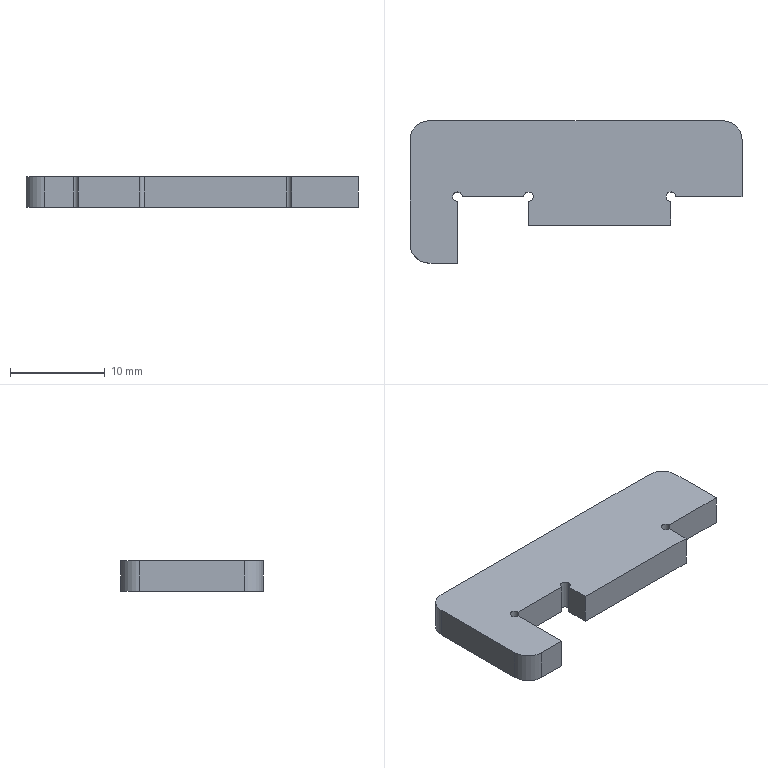Part | SolidWorks | features Fillet 1, FlatPattern 1, SMBaseFlange 1, SheetMetal 1 | 1 solid | 19 faces | box 35 x 15 x 3.2 mm | volume 1138 mm3 | plane 12 | cylinder 7 | commonest cylinder face diameters 1 x4 4 x3
STEP:
#1=CARTESIAN_POINT('',(47.21,-235.,-3.2));
#2=VERTEX_POINT('',#1);
#3=CARTESIAN_POINT('',(48.21,-235.,-3.2));
#4=VERTEX_POINT('',#3);
#5=CARTESIAN_POINT('',(47.71,-235.,-3.2));
#6=DIRECTION('',(0.,0.,-1.));
#7=DIRECTION('',(1.,0.,0.));
#8=AXIS2_PLACEMENT_3D('',#5,#6,#7);
#9=CIRCLE('',#8,0.5);
#10=EDGE_CURVE('',#2,#4,#9,.T.);
#11=ORIENTED_EDGE('',*,*,#10,.T.);
#12=CARTESIAN_POINT('',(48.21,-235.,0.));
#13=VERTEX_POINT('',#12);
#14=CARTESIAN_POINT('',(48.21,-235.,-3.2));
#15=DIRECTION('',(0.,0.,1.));
#16=VECTOR('',#15,1000.);
#17=LINE('',#14,#16);
#18=EDGE_CURVE('',#4,#13,#17,.T.);
#19=ORIENTED_EDGE('',*,*,#18,.T.);
#20=CARTESIAN_POINT('',(47.21,-235.,0.));
#21=VERTEX_POINT('',#20);
#22=CARTESIAN_POINT('',(47.71,-235.,0.));
#23=DIRECTION('',(0.,0.,-1.));
#24=DIRECTION('',(1.,0.,0.));
#25=AXIS2_PLACEMENT_3D('',#22,#23,#24);
#26=CIRCLE('',#25,0.5);
#27=EDGE_CURVE('',#21,#13,#26,.T.);
#28=ORIENTED_EDGE('',*,*,#27,.F.);
#29=CARTESIAN_POINT('',(47.21,-235.,-3.2));
#30=DIRECTION('',(0.,0.,1.));
#31=VECTOR('',#30,1000.);
#32=LINE('',#29,#31);
#33=EDGE_CURVE('',#2,#21,#32,.T.);
#34=ORIENTED_EDGE('',*,*,#33,.F.);
#35=EDGE_LOOP('',(#11,#19,#28,#34));
#36=FACE_OUTER_BOUND('',#35,.T.);
#37=CARTESIAN_POINT('',(47.71,-235.,-3.2));
#38=DIRECTION('',(0.,0.,1.));
#39=DIRECTION('',(1.,0.,0.));
#40=AXIS2_PLACEMENT_3D('',#37,#38,#39);
#41=CYLINDRICAL_SURFACE('',#40,0.5);
#42=ADVANCED_FACE('',(#36),#41,.F.);
#43=CARTESIAN_POINT('',(37.21,-242.,0.));
#44=VERTEX_POINT('',#43);
#45=CARTESIAN_POINT('',(40.21,-242.,0.));
#46=VERTEX_POINT('',#45);
#47=CARTESIAN_POINT('',(40.21,-242.,0.));
#48=DIRECTION('',(1.,0.,0.));
#49=VECTOR('',#48,1000.);
#50=LINE('',#47,#49);
#51=EDGE_CURVE('',#44,#46,#50,.T.);
#52=ORIENTED_EDGE('',*,*,#51,.F.);
#53=CARTESIAN_POINT('',(37.21,-242.,-3.2));
#54=VERTEX_POINT('',#53);
#55=CARTESIAN_POINT('',(37.21,-242.,-3.2));
#56=DIRECTION('',(0.,0.,-1.));
#57=VECTOR('',#56,1000.);
#58=LINE('',#55,#57);
#59=EDGE_CURVE('',#44,#54,#58,.T.);
#60=ORIENTED_EDGE('',*,*,#59,.T.);
#61=CARTESIAN_POINT('',(40.21,-242.,-3.2));
#62=VERTEX_POINT('',#61);
#63=CARTESIAN_POINT('',(40.21,-242.,-3.2));
#64=DIRECTION('',(1.,0.,0.));
#65=VECTOR('',#64,1000.);
#66=LINE('',#63,#65);
#67=EDGE_CURVE('',#54,#62,#66,.T.);
#68=ORIENTED_EDGE('',*,*,#67,.T.);
#69=CARTESIAN_POINT('',(40.21,-242.,-3.2));
#70=DIRECTION('',(0.,0.,1.));
#71=VECTOR('',#70,1000.);
#72=LINE('',#69,#71);
#73=EDGE_CURVE('',#62,#46,#72,.T.);
#74=ORIENTED_EDGE('',*,*,#73,.T.);
#75=EDGE_LOOP('',(#52,#60,#68,#74));
#76=FACE_OUTER_BOUND('',#75,.T.);
#77=CARTESIAN_POINT('',(40.21,-242.,-3.2));
#78=DIRECTION('',(0.,-1.,0.));
#79=DIRECTION('',(0.,0.,-1.));
#80=AXIS2_PLACEMENT_3D('',#77,#78,#79);
#81=PLANE('',#80);
#82=ADVANCED_FACE('',(#76),#81,.T.);
#83=CARTESIAN_POINT('',(35.21,-229.,0.));
#84=VERTEX_POINT('',#83);
#85=CARTESIAN_POINT('',(35.21,-240.,0.));
#86=VERTEX_POINT('',#85);
#87=CARTESIAN_POINT('',(35.21,-242.,0.));
#88=DIRECTION('',(0.,-1.,0.));
#89=VECTOR('',#88,1000.);
#90=LINE('',#87,#89);
#91=EDGE_CURVE('',#84,#86,#90,.T.);
#92=ORIENTED_EDGE('',*,*,#91,.F.);
#93=CARTESIAN_POINT('',(35.21,-229.,-3.2));
#94=VERTEX_POINT('',#93);
#95=CARTESIAN_POINT('',(35.21,-229.,-3.2));
#96=DIRECTION('',(0.,0.,-1.));
#97=VECTOR('',#96,1000.);
#98=LINE('',#95,#97);
#99=EDGE_CURVE('',#84,#94,#98,.T.);
#100=ORIENTED_EDGE('',*,*,#99,.T.);
#101=CARTESIAN_POINT('',(35.21,-240.,-3.2));
#102=VERTEX_POINT('',#101);
#103=CARTESIAN_POINT('',(35.21,-242.,-3.2));
#104=DIRECTION('',(0.,-1.,0.));
#105=VECTOR('',#104,1000.);
#106=LINE('',#103,#105);
#107=EDGE_CURVE('',#94,#102,#106,.T.);
#108=ORIENTED_EDGE('',*,*,#107,.T.);
#109=CARTESIAN_POINT('',(35.21,-240.,-3.2));
#110=DIRECTION('',(0.,0.,1.));
#111=VECTOR('',#110,1000.);
#112=LINE('',#109,#111);
#113=EDGE_CURVE('',#102,#86,#112,.T.);
#114=ORIENTED_EDGE('',*,*,#113,.T.);
#115=EDGE_LOOP('',(#92,#100,#108,#114));
#116=FACE_OUTER_BOUND('',#115,.T.);
#117=CARTESIAN_POINT('',(35.21,-242.,-3.2));
#118=DIRECTION('',(-1.,0.,0.));
#119=DIRECTION('',(0.,0.,1.));
#120=AXIS2_PLACEMENT_3D('',#117,#118,#119);
#121=PLANE('',#120);
#122=ADVANCED_FACE('',(#116),#121,.T.);
#123=CARTESIAN_POINT('',(68.21,-227.,0.));
#124=VERTEX_POINT('',#123);
#125=CARTESIAN_POINT('',(37.21,-227.,0.));
#126=VERTEX_POINT('',#125);
#127=CARTESIAN_POINT('',(35.21,-227.,0.));
#128=DIRECTION('',(-1.,0.,0.));
#129=VECTOR('',#128,1000.);
#130=LINE('',#127,#129);
#131=EDGE_CURVE('',#124,#126,#130,.T.);
#132=ORIENTED_EDGE('',*,*,#131,.F.);
#133=CARTESIAN_POINT('',(68.21,-227.,-3.2));
#134=VERTEX_POINT('',#133);
#135=CARTESIAN_POINT('',(68.21,-227.,-3.2));
#136=DIRECTION('',(0.,0.,-1.));
#137=VECTOR('',#136,1000.);
#138=LINE('',#135,#137);
#139=EDGE_CURVE('',#124,#134,#138,.T.);
#140=ORIENTED_EDGE('',*,*,#139,.T.);
#141=CARTESIAN_POINT('',(37.21,-227.,-3.2));
#142=VERTEX_POINT('',#141);
#143=CARTESIAN_POINT('',(35.21,-227.,-3.2));
#144=DIRECTION('',(-1.,0.,0.));
#145=VECTOR('',#144,1000.);
#146=LINE('',#143,#145);
#147=EDGE_CURVE('',#134,#142,#146,.T.);
#148=ORIENTED_EDGE('',*,*,#147,.T.);
#149=CARTESIAN_POINT('',(37.21,-227.,-3.2));
#150=DIRECTION('',(0.,0.,1.));
#151=VECTOR('',#150,1000.);
#152=LINE('',#149,#151);
#153=EDGE_CURVE('',#142,#126,#152,.T.);
#154=ORIENTED_EDGE('',*,*,#153,.T.);
#155=EDGE_LOOP('',(#132,#140,#148,#154));
#156=FACE_OUTER_BOUND('',#155,.T.);
#157=CARTESIAN_POINT('',(35.21,-227.,-3.2));
#158=DIRECTION('',(0.,1.,0.));
#159=DIRECTION('',(0.,0.,1.));
#160=AXIS2_PLACEMENT_3D('',#157,#158,#159);
#161=PLANE('',#160);
#162=ADVANCED_FACE('',(#156),#161,.T.);
#163=CARTESIAN_POINT('',(70.21,-235.,-3.2));
#164=VERTEX_POINT('',#163);
#165=CARTESIAN_POINT('',(70.21,-229.,-3.2));
#166=VERTEX_POINT('',#165);
#167=CARTESIAN_POINT('',(70.21,-227.,-3.2));
#168=DIRECTION('',(0.,1.,0.));
#169=VECTOR('',#168,1000.);
#170=LINE('',#167,#169);
#171=EDGE_CURVE('',#164,#166,#170,.T.);
#172=ORIENTED_EDGE('',*,*,#171,.T.);
#173=CARTESIAN_POINT('',(70.21,-229.,0.));
#174=VERTEX_POINT('',#173);
#175=CARTESIAN_POINT('',(70.21,-229.,-3.2));
#176=DIRECTION('',(0.,0.,1.));
#177=VECTOR('',#176,1000.);
#178=LINE('',#175,#177);
#179=EDGE_CURVE('',#166,#174,#178,.T.);
#180=ORIENTED_EDGE('',*,*,#179,.T.);
#181=CARTESIAN_POINT('',(70.21,-235.,0.));
#182=VERTEX_POINT('',#181);
#183=CARTESIAN_POINT('',(70.21,-227.,0.));
#184=DIRECTION('',(0.,1.,0.));
#185=VECTOR('',#184,1000.);
#186=LINE('',#183,#185);
#187=EDGE_CURVE('',#182,#174,#186,.T.);
#188=ORIENTED_EDGE('',*,*,#187,.F.);
#189=CARTESIAN_POINT('',(70.21,-235.,-3.2));
#190=DIRECTION('',(0.,0.,1.));
#191=VECTOR('',#190,1000.);
#192=LINE('',#189,#191);
#193=EDGE_CURVE('',#164,#182,#192,.T.);
#194=ORIENTED_EDGE('',*,*,#193,.F.);
#195=EDGE_LOOP('',(#172,#180,#188,#194));
#196=FACE_OUTER_BOUND('',#195,.T.);
#197=CARTESIAN_POINT('',(70.21,-227.,-3.2));
#198=DIRECTION('',(1.,0.,0.));
#199=DIRECTION('',(0.,0.,-1.));
#200=AXIS2_PLACEMENT_3D('',#197,#198,#199);
#201=PLANE('',#200);
#202=ADVANCED_FACE('',(#196),#201,.T.);
#203=CARTESIAN_POINT('',(63.21,-235.,0.));
#204=VERTEX_POINT('',#203);
#205=CARTESIAN_POINT('',(70.21,-235.,0.));
#206=DIRECTION('',(1.,0.,0.));
#207=VECTOR('',#206,1000.);
#208=LINE('',#205,#207);
#209=EDGE_CURVE('',#204,#182,#208,.T.);
#210=ORIENTED_EDGE('',*,*,#209,.F.);
#211=CARTESIAN_POINT('',(63.21,-235.,-3.2));
#212=VERTEX_POINT('',#211);
#213=CARTESIAN_POINT('',(63.21,-235.,-3.2));
#214=DIRECTION('',(0.,0.,1.));
#215=VECTOR('',#214,1000.);
#216=LINE('',#213,#215);
#217=EDGE_CURVE('',#212,#204,#216,.T.);
#218=ORIENTED_EDGE('',*,*,#217,.F.);
#219=CARTESIAN_POINT('',(70.21,-235.,-3.2));
#220=DIRECTION('',(1.,0.,0.));
#221=VECTOR('',#220,1000.);
#222=LINE('',#219,#221);
#223=EDGE_CURVE('',#212,#164,#222,.T.);
#224=ORIENTED_EDGE('',*,*,#223,.T.);
#225=ORIENTED_EDGE('',*,*,#193,.T.);
#226=EDGE_LOOP('',(#210,#218,#224,#225));
#227=FACE_OUTER_BOUND('',#226,.T.);
#228=CARTESIAN_POINT('',(70.21,-235.,-3.2));
#229=DIRECTION('',(0.,-1.,0.));
#230=DIRECTION('',(0.,0.,-1.));
#231=AXIS2_PLACEMENT_3D('',#228,#229,#230);
#232=PLANE('',#231);
#233=ADVANCED_FACE('',(#227),#232,.T.);
#234=CARTESIAN_POINT('',(62.71,-235.5,0.));
#235=VERTEX_POINT('',#234);
#236=CARTESIAN_POINT('',(62.71,-235.,0.));
#237=DIRECTION('',(0.,0.,-1.));
#238=DIRECTION('',(1.,0.,0.));
#239=AXIS2_PLACEMENT_3D('',#236,#237,#238);
#240=CIRCLE('',#239,0.5);
#241=EDGE_CURVE('',#235,#204,#240,.T.);
#242=ORIENTED_EDGE('',*,*,#241,.F.);
#243=CARTESIAN_POINT('',(62.71,-235.5,-3.2));
#244=VERTEX_POINT('',#243);
#245=CARTESIAN_POINT('',(62.71,-235.5,-3.2));
#246=DIRECTION('',(0.,0.,1.));
#247=VECTOR('',#246,1000.);
#248=LINE('',#245,#247);
#249=EDGE_CURVE('',#244,#235,#248,.T.);
#250=ORIENTED_EDGE('',*,*,#249,.F.);
#251=CARTESIAN_POINT('',(62.71,-235.,-3.2));
#252=DIRECTION('',(0.,0.,-1.));
#253=DIRECTION('',(1.,0.,0.));
#254=AXIS2_PLACEMENT_3D('',#251,#252,#253);
#255=CIRCLE('',#254,0.5);
#256=EDGE_CURVE('',#244,#212,#255,.T.);
#257=ORIENTED_EDGE('',*,*,#256,.T.);
#258=ORIENTED_EDGE('',*,*,#217,.T.);
#259=EDGE_LOOP('',(#242,#250,#257,#258));
#260=FACE_OUTER_BOUND('',#259,.T.);
#261=CARTESIAN_POINT('',(62.71,-235.,-3.2));
#262=DIRECTION('',(0.,0.,1.));
#263=DIRECTION('',(1.,0.,0.));
#264=AXIS2_PLACEMENT_3D('',#261,#262,#263);
#265=CYLINDRICAL_SURFACE('',#264,0.5);
#266=ADVANCED_FACE('',(#260),#265,.F.);
#267=CARTESIAN_POINT('',(62.71,-238.,0.));
#268=VERTEX_POINT('',#267);
#269=CARTESIAN_POINT('',(62.71,-235.5,0.));
#270=DIRECTION('',(0.,1.,0.));
#271=VECTOR('',#270,1000.);
#272=LINE('',#269,#271);
#273=EDGE_CURVE('',#268,#235,#272,.T.);
#274=ORIENTED_EDGE('',*,*,#273,.F.);
#275=CARTESIAN_POINT('',(62.71,-238.,-3.2));
#276=VERTEX_POINT('',#275);
#277=CARTESIAN_POINT('',(62.71,-238.,-3.2));
#278=DIRECTION('',(0.,0.,1.));
#279=VECTOR('',#278,1000.);
#280=LINE('',#277,#279);
#281=EDGE_CURVE('',#276,#268,#280,.T.);
#282=ORIENTED_EDGE('',*,*,#281,.F.);
#283=CARTESIAN_POINT('',(62.71,-235.5,-3.2));
#284=DIRECTION('',(0.,1.,0.));
#285=VECTOR('',#284,1000.);
#286=LINE('',#283,#285);
#287=EDGE_CURVE('',#276,#244,#286,.T.);
#288=ORIENTED_EDGE('',*,*,#287,.T.);
#289=ORIENTED_EDGE('',*,*,#249,.T.);
#290=EDGE_LOOP('',(#274,#282,#288,#289));
#291=FACE_OUTER_BOUND('',#290,.T.);
#292=CARTESIAN_POINT('',(62.71,-235.5,-3.2));
#293=DIRECTION('',(1.,0.,0.));
#294=DIRECTION('',(0.,0.,-1.));
#295=AXIS2_PLACEMENT_3D('',#292,#293,#294);
#296=PLANE('',#295);
#297=ADVANCED_FACE('',(#291),#296,.T.);
#298=CARTESIAN_POINT('',(47.71,-238.,0.));
#299=VERTEX_POINT('',#298);
#300=CARTESIAN_POINT('',(62.71,-238.,0.));
#301=DIRECTION('',(1.,0.,0.));
#302=VECTOR('',#301,1000.);
#303=LINE('',#300,#302);
#304=EDGE_CURVE('',#299,#268,#303,.T.);
#305=ORIENTED_EDGE('',*,*,#304,.F.);
#306=CARTESIAN_POINT('',(47.71,-238.,-3.2));
#307=VERTEX_POINT('',#306);
#308=CARTESIAN_POINT('',(47.71,-238.,-3.2));
#309=DIRECTION('',(0.,0.,1.));
#310=VECTOR('',#309,1000.);
#311=LINE('',#308,#310);
#312=EDGE_CURVE('',#307,#299,#311,.T.);
#313=ORIENTED_EDGE('',*,*,#312,.F.);
#314=CARTESIAN_POINT('',(62.71,-238.,-3.2));
#315=DIRECTION('',(1.,0.,0.));
#316=VECTOR('',#315,1000.);
#317=LINE('',#314,#316);
#318=EDGE_CURVE('',#307,#276,#317,.T.);
#319=ORIENTED_EDGE('',*,*,#318,.T.);
#320=ORIENTED_EDGE('',*,*,#281,.T.);
#321=EDGE_LOOP('',(#305,#313,#319,#320));
#322=FACE_OUTER_BOUND('',#321,.T.);
#323=CARTESIAN_POINT('',(62.71,-238.,-3.2));
#324=DIRECTION('',(0.,-1.,0.));
#325=DIRECTION('',(1.,0.,0.));
#326=AXIS2_PLACEMENT_3D('',#323,#324,#325);
#327=PLANE('',#326);
#328=ADVANCED_FACE('',(#322),#327,.T.);
#329=CARTESIAN_POINT('',(47.71,-235.5,0.));
#330=VERTEX_POINT('',#329);
#331=CARTESIAN_POINT('',(47.71,-238.,0.));
#332=DIRECTION('',(0.,-1.,0.));
#333=VECTOR('',#332,1000.);
#334=LINE('',#331,#333);
#335=EDGE_CURVE('',#330,#299,#334,.T.);
#336=ORIENTED_EDGE('',*,*,#335,.F.);
#337=CARTESIAN_POINT('',(47.71,-235.5,-3.2));
#338=VERTEX_POINT('',#337);
#339=CARTESIAN_POINT('',(47.71,-235.5,-3.2));
#340=DIRECTION('',(0.,0.,1.));
#341=VECTOR('',#340,1000.);
#342=LINE('',#339,#341);
#343=EDGE_CURVE('',#338,#330,#342,.T.);
#344=ORIENTED_EDGE('',*,*,#343,.F.);
#345=CARTESIAN_POINT('',(47.71,-238.,-3.2));
#346=DIRECTION('',(0.,-1.,0.));
#347=VECTOR('',#346,1000.);
#348=LINE('',#345,#347);
#349=EDGE_CURVE('',#338,#307,#348,.T.);
#350=ORIENTED_EDGE('',*,*,#349,.T.);
#351=ORIENTED_EDGE('',*,*,#312,.T.);
#352=EDGE_LOOP('',(#336,#344,#350,#351));
#353=FACE_OUTER_BOUND('',#352,.T.);
#354=CARTESIAN_POINT('',(47.71,-238.,-3.2));
#355=DIRECTION('',(-1.,0.,0.));
#356=DIRECTION('',(0.,0.,1.));
#357=AXIS2_PLACEMENT_3D('',#354,#355,#356);
#358=PLANE('',#357);
#359=ADVANCED_FACE('',(#353),#358,.T.);
#360=ORIENTED_EDGE('',*,*,#18,.F.);
#361=CARTESIAN_POINT('',(47.71,-235.,-3.2));
#362=DIRECTION('',(0.,0.,-1.));
#363=DIRECTION('',(1.,0.,0.));
#364=AXIS2_PLACEMENT_3D('',#361,#362,#363);
#365=CIRCLE('',#364,0.5);
#366=EDGE_CURVE('',#4,#338,#365,.T.);
#367=ORIENTED_EDGE('',*,*,#366,.T.);
#368=ORIENTED_EDGE('',*,*,#343,.T.);
#369=CARTESIAN_POINT('',(47.71,-235.,0.));
#370=DIRECTION('',(0.,0.,-1.));
#371=DIRECTION('',(1.,0.,0.));
#372=AXIS2_PLACEMENT_3D('',#369,#370,#371);
#373=CIRCLE('',#372,0.5);
#374=EDGE_CURVE('',#13,#330,#373,.T.);
#375=ORIENTED_EDGE('',*,*,#374,.F.);
#376=EDGE_LOOP('',(#360,#367,#368,#375));
#377=FACE_OUTER_BOUND('',#376,.T.);
#378=CARTESIAN_POINT('',(47.71,-235.,-3.2));
#379=DIRECTION('',(0.,0.,1.));
#380=DIRECTION('',(1.,0.,0.));
#381=AXIS2_PLACEMENT_3D('',#378,#379,#380);
#382=CYLINDRICAL_SURFACE('',#381,0.5);
#383=ADVANCED_FACE('',(#377),#382,.F.);
#384=CARTESIAN_POINT('',(40.71,-235.,0.));
#385=VERTEX_POINT('',#384);
#386=CARTESIAN_POINT('',(47.21,-235.,0.));
#387=DIRECTION('',(1.,0.,0.));
#388=VECTOR('',#387,1000.);
#389=LINE('',#386,#388);
#390=EDGE_CURVE('',#385,#21,#389,.T.);
#391=ORIENTED_EDGE('',*,*,#390,.F.);
#392=CARTESIAN_POINT('',(40.71,-235.,-3.2));
#393=VERTEX_POINT('',#392);
#394=CARTESIAN_POINT('',(40.71,-235.,-3.2));
#395=DIRECTION('',(0.,0.,1.));
#396=VECTOR('',#395,1000.);
#397=LINE('',#394,#396);
#398=EDGE_CURVE('',#393,#385,#397,.T.);
#399=ORIENTED_EDGE('',*,*,#398,.F.);
#400=CARTESIAN_POINT('',(47.21,-235.,-3.2));
#401=DIRECTION('',(1.,0.,0.));
#402=VECTOR('',#401,1000.);
#403=LINE('',#400,#402);
#404=EDGE_CURVE('',#393,#2,#403,.T.);
#405=ORIENTED_EDGE('',*,*,#404,.T.);
#406=ORIENTED_EDGE('',*,*,#33,.T.);
#407=EDGE_LOOP('',(#391,#399,#405,#406));
#408=FACE_OUTER_BOUND('',#407,.T.);
#409=CARTESIAN_POINT('',(47.21,-235.,-3.2));
#410=DIRECTION('',(0.,-1.,0.));
#411=DIRECTION('',(0.,0.,-1.));
#412=AXIS2_PLACEMENT_3D('',#409,#410,#411);
#413=PLANE('',#412);
#414=ADVANCED_FACE('',(#408),#413,.T.);
#415=CARTESIAN_POINT('',(40.21,-235.5,0.));
#416=VERTEX_POINT('',#415);
#417=CARTESIAN_POINT('',(40.21,-235.,0.));
#418=DIRECTION('',(0.,0.,-1.));
#419=DIRECTION('',(1.,0.,0.));
#420=AXIS2_PLACEMENT_3D('',#417,#418,#419);
#421=CIRCLE('',#420,0.5);
#422=EDGE_CURVE('',#416,#385,#421,.T.);
#423=ORIENTED_EDGE('',*,*,#422,.F.);
#424=CARTESIAN_POINT('',(40.21,-235.5,-3.2));
#425=VERTEX_POINT('',#424);
#426=CARTESIAN_POINT('',(40.21,-235.5,-3.2));
#427=DIRECTION('',(0.,0.,1.));
#428=VECTOR('',#427,1000.);
#429=LINE('',#426,#428);
#430=EDGE_CURVE('',#425,#416,#429,.T.);
#431=ORIENTED_EDGE('',*,*,#430,.F.);
#432=CARTESIAN_POINT('',(40.21,-235.,-3.2));
#433=DIRECTION('',(0.,0.,-1.));
#434=DIRECTION('',(1.,0.,0.));
#435=AXIS2_PLACEMENT_3D('',#432,#433,#434);
#436=CIRCLE('',#435,0.5);
#437=EDGE_CURVE('',#425,#393,#436,.T.);
#438=ORIENTED_EDGE('',*,*,#437,.T.);
#439=ORIENTED_EDGE('',*,*,#398,.T.);
#440=EDGE_LOOP('',(#423,#431,#438,#439));
#441=FACE_OUTER_BOUND('',#440,.T.);
#442=CARTESIAN_POINT('',(40.21,-235.,-3.2));
#443=DIRECTION('',(0.,0.,1.));
#444=DIRECTION('',(1.,0.,0.));
#445=AXIS2_PLACEMENT_3D('',#442,#443,#444);
#446=CYLINDRICAL_SURFACE('',#445,0.5);
#447=ADVANCED_FACE('',(#441),#446,.F.);
#448=CARTESIAN_POINT('',(40.21,-235.5,0.));
#449=DIRECTION('',(0.,1.,0.));
#450=VECTOR('',#449,1000.);
#451=LINE('',#448,#450);
#452=EDGE_CURVE('',#46,#416,#451,.T.);
#453=ORIENTED_EDGE('',*,*,#452,.F.);
#454=ORIENTED_EDGE('',*,*,#73,.F.);
#455=CARTESIAN_POINT('',(40.21,-235.5,-3.2));
#456=DIRECTION('',(0.,1.,0.));
#457=VECTOR('',#456,1000.);
#458=LINE('',#455,#457);
#459=EDGE_CURVE('',#62,#425,#458,.T.);
#460=ORIENTED_EDGE('',*,*,#459,.T.);
#461=ORIENTED_EDGE('',*,*,#430,.T.);
#462=EDGE_LOOP('',(#453,#454,#460,#461));
#463=FACE_OUTER_BOUND('',#462,.T.);
#464=CARTESIAN_POINT('',(40.21,-235.5,-3.2));
#465=DIRECTION('',(1.,0.,0.));
#466=DIRECTION('',(0.,0.,-1.));
#467=AXIS2_PLACEMENT_3D('',#464,#465,#466);
#468=PLANE('',#467);
#469=ADVANCED_FACE('',(#463),#468,.T.);
#470=ORIENTED_EDGE('',*,*,#147,.F.);
#471=CARTESIAN_POINT('',(68.21,-229.,-3.2));
#472=DIRECTION('',(0.,0.,-1.));
#473=DIRECTION('',(1.,0.,0.));
#474=AXIS2_PLACEMENT_3D('',#471,#472,#473);
#475=CIRCLE('',#474,2.);
#476=EDGE_CURVE('',#134,#166,#475,.T.);
#477=ORIENTED_EDGE('',*,*,#476,.T.);
#478=ORIENTED_EDGE('',*,*,#171,.F.);
#479=ORIENTED_EDGE('',*,*,#223,.F.);
#480=ORIENTED_EDGE('',*,*,#256,.F.);
#481=ORIENTED_EDGE('',*,*,#287,.F.);
#482=ORIENTED_EDGE('',*,*,#318,.F.);
#483=ORIENTED_EDGE('',*,*,#349,.F.);
#484=ORIENTED_EDGE('',*,*,#366,.F.);
#485=ORIENTED_EDGE('',*,*,#10,.F.);
#486=ORIENTED_EDGE('',*,*,#404,.F.);
#487=ORIENTED_EDGE('',*,*,#437,.F.);
#488=ORIENTED_EDGE('',*,*,#459,.F.);
#489=ORIENTED_EDGE('',*,*,#67,.F.);
#490=CARTESIAN_POINT('',(37.21,-240.,-3.2));
#491=DIRECTION('',(0.,0.,-1.));
#492=DIRECTION('',(1.,0.,0.));
#493=AXIS2_PLACEMENT_3D('',#490,#491,#492);
#494=CIRCLE('',#493,2.);
#495=EDGE_CURVE('',#54,#102,#494,.T.);
#496=ORIENTED_EDGE('',*,*,#495,.T.);
#497=ORIENTED_EDGE('',*,*,#107,.F.);
#498=CARTESIAN_POINT('',(37.21,-229.,-3.2));
#499=DIRECTION('',(0.,0.,-1.));
#500=DIRECTION('',(1.,0.,0.));
#501=AXIS2_PLACEMENT_3D('',#498,#499,#500);
#502=CIRCLE('',#501,2.);
#503=EDGE_CURVE('',#94,#142,#502,.T.);
#504=ORIENTED_EDGE('',*,*,#503,.T.);
#505=EDGE_LOOP('',(#470,#477,#478,#479,#480,#481,#482,#483,#484,#485,#486,#487,#488,#489,#496,#497,#504));
#506=FACE_OUTER_BOUND('',#505,.T.);
#507=CARTESIAN_POINT('',(62.71,-235.,-3.2));
#508=DIRECTION('',(0.,0.,1.));
#509=DIRECTION('',(1.,0.,0.));
#510=AXIS2_PLACEMENT_3D('',#507,#508,#509);
#511=PLANE('',#510);
#512=ADVANCED_FACE('',(#506),#511,.F.);
#513=ORIENTED_EDGE('',*,*,#187,.T.);
#514=CARTESIAN_POINT('',(68.21,-229.,0.));
#515=DIRECTION('',(0.,0.,1.));
#516=DIRECTION('',(1.,0.,0.));
#517=AXIS2_PLACEMENT_3D('',#514,#515,#516);
#518=CIRCLE('',#517,2.);
#519=EDGE_CURVE('',#174,#124,#518,.T.);
#520=ORIENTED_EDGE('',*,*,#519,.T.);
#521=ORIENTED_EDGE('',*,*,#131,.T.);
#522=CARTESIAN_POINT('',(37.21,-229.,0.));
#523=DIRECTION('',(0.,0.,1.));
#524=DIRECTION('',(1.,0.,0.));
#525=AXIS2_PLACEMENT_3D('',#522,#523,#524);
#526=CIRCLE('',#525,2.);
#527=EDGE_CURVE('',#126,#84,#526,.T.);
#528=ORIENTED_EDGE('',*,*,#527,.T.);
#529=ORIENTED_EDGE('',*,*,#91,.T.);
#530=CARTESIAN_POINT('',(37.21,-240.,0.));
#531=DIRECTION('',(0.,0.,1.));
#532=DIRECTION('',(1.,0.,0.));
#533=AXIS2_PLACEMENT_3D('',#530,#531,#532);
#534=CIRCLE('',#533,2.);
#535=EDGE_CURVE('',#86,#44,#534,.T.);
#536=ORIENTED_EDGE('',*,*,#535,.T.);
#537=ORIENTED_EDGE('',*,*,#51,.T.);
#538=ORIENTED_EDGE('',*,*,#452,.T.);
#539=ORIENTED_EDGE('',*,*,#422,.T.);
#540=ORIENTED_EDGE('',*,*,#390,.T.);
#541=ORIENTED_EDGE('',*,*,#27,.T.);
#542=ORIENTED_EDGE('',*,*,#374,.T.);
#543=ORIENTED_EDGE('',*,*,#335,.T.);
#544=ORIENTED_EDGE('',*,*,#304,.T.);
#545=ORIENTED_EDGE('',*,*,#273,.T.);
#546=ORIENTED_EDGE('',*,*,#241,.T.);
#547=ORIENTED_EDGE('',*,*,#209,.T.);
#548=EDGE_LOOP('',(#513,#520,#521,#528,#529,#536,#537,#538,#539,#540,#541,#542,#543,#544,#545,#546,#547));
#549=FACE_OUTER_BOUND('',#548,.T.);
#550=CARTESIAN_POINT('',(62.71,-235.,0.));
#551=DIRECTION('',(0.,0.,1.));
#552=DIRECTION('',(1.,0.,0.));
#553=AXIS2_PLACEMENT_3D('',#550,#551,#552);
#554=PLANE('',#553);
#555=ADVANCED_FACE('',(#549),#554,.T.);
#556=ORIENTED_EDGE('',*,*,#476,.F.);
#557=ORIENTED_EDGE('',*,*,#139,.F.);
#558=ORIENTED_EDGE('',*,*,#519,.F.);
#559=ORIENTED_EDGE('',*,*,#179,.F.);
#560=EDGE_LOOP('',(#556,#557,#558,#559));
#561=FACE_OUTER_BOUND('',#560,.T.);
#562=CARTESIAN_POINT('',(68.21,-229.,-3.2));
#563=DIRECTION('',(0.,0.,1.));
#564=DIRECTION('',(1.,0.,0.));
#565=AXIS2_PLACEMENT_3D('',#562,#563,#564);
#566=CYLINDRICAL_SURFACE('',#565,2.);
#567=ADVANCED_FACE('',(#561),#566,.T.);
#568=ORIENTED_EDGE('',*,*,#503,.F.);
#569=ORIENTED_EDGE('',*,*,#99,.F.);
#570=ORIENTED_EDGE('',*,*,#527,.F.);
#571=ORIENTED_EDGE('',*,*,#153,.F.);
#572=EDGE_LOOP('',(#568,#569,#570,#571));
#573=FACE_OUTER_BOUND('',#572,.T.);
#574=CARTESIAN_POINT('',(37.21,-229.,-3.2));
#575=DIRECTION('',(0.,0.,1.));
#576=DIRECTION('',(1.,0.,0.));
#577=AXIS2_PLACEMENT_3D('',#574,#575,#576);
#578=CYLINDRICAL_SURFACE('',#577,2.);
#579=ADVANCED_FACE('',(#573),#578,.T.);
#580=ORIENTED_EDGE('',*,*,#495,.F.);
#581=ORIENTED_EDGE('',*,*,#59,.F.);
#582=ORIENTED_EDGE('',*,*,#535,.F.);
#583=ORIENTED_EDGE('',*,*,#113,.F.);
#584=EDGE_LOOP('',(#580,#581,#582,#583));
#585=FACE_OUTER_BOUND('',#584,.T.);
#586=CARTESIAN_POINT('',(37.21,-240.,-3.2));
#587=DIRECTION('',(0.,0.,1.));
#588=DIRECTION('',(1.,0.,0.));
#589=AXIS2_PLACEMENT_3D('',#586,#587,#588);
#590=CYLINDRICAL_SURFACE('',#589,2.);
#591=ADVANCED_FACE('',(#585),#590,.T.);
#592=CLOSED_SHELL('',(#42,#82,#122,#162,#202,#233,#266,#297,#328,#359,#383,#414,#447,#469,#512,#555,#567,#579,#591));
#593=MANIFOLD_SOLID_BREP('',#592);
#594=CARTESIAN_POINT('',(0.,0.,0.));
#595=DIRECTION('',(0.,0.,1.));
#596=DIRECTION('',(1.,0.,0.));
#597=AXIS2_PLACEMENT_3D('',#594,#595,#596);
#598=(LENGTH_UNIT()NAMED_UNIT(*)SI_UNIT(.MILLI.,.METRE.));
#599=UNCERTAINTY_MEASURE_WITH_UNIT(LENGTH_MEASURE(0.00001),#598,'','');
#600=(NAMED_UNIT(*)PLANE_ANGLE_UNIT()SI_UNIT($,.RADIAN.));
#601=(NAMED_UNIT(*)SI_UNIT($,.STERADIAN.)SOLID_ANGLE_UNIT());
#602=(GEOMETRIC_REPRESENTATION_CONTEXT(3)GLOBAL_UNCERTAINTY_ASSIGNED_CONTEXT((#599))GLOBAL_UNIT_ASSIGNED_CONTEXT((#598,#600,#601))REPRESENTATION_CONTEXT('',''));
#603=ADVANCED_BREP_SHAPE_REPRESENTATION('',(#593,#597),#602);